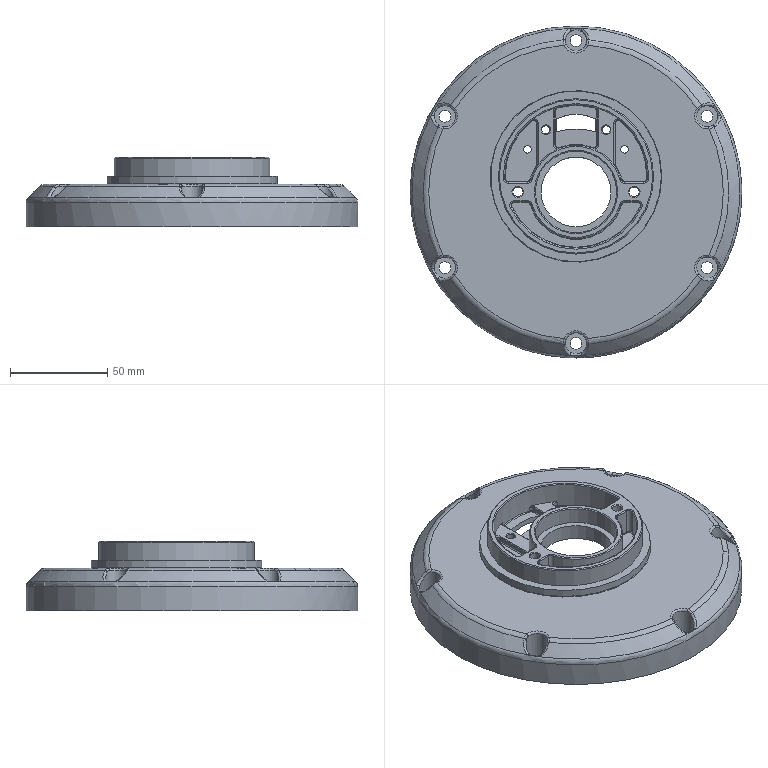NC program | NX | posted with a generic post | part box 171 x 171 x 36 mm
Lines 26826 to 27758 of 127321:
(3D开粗_COPY_COPY , TOOL : D4-L24)
N53638 T08 M6
N53640 G54
N53642 G17 G0 G90 X-30.607 Y7.686 S5000 M3
N53644 G43 Z20. H8
N53646 Z0.152
N53648 G94 G1 Z-0.148 F2500.
N53650 Y7.65
N53652 G3 X-30.007 Y7.05 R0.6
N53654 G1 X-25.078
N53656 G2 X25.078 Y7.05 R26.05
N53658 G1 X34.937
N53660 G3 X-34.937 Y7.05 R-34.95
N53662 G1 X-30.007
N53664 X-29.507
N53666 G3 X-28.907 Y7.65 R0.6
N53668 G1 Y7.686
N53670 Z0.152
N53672 X-30.607 Y7.74 Z0.004 F15000.
N53674 Z-0.296 F2500.
N53676 Y7.725
N53678 G3 X-30.007 Y7.125 R0.6
N53680 G1 X-25.135
N53682 G2 X25.135 Y7.125 R26.125
N53684 G1 X34.864
N53686 G3 X-34.864 Y7.125 R-34.875
N53688 G1 X-30.007
N53690 X-29.507
N53692 G3 X-28.907 Y7.73 R0.6
N53694 G1 Z0.004
N53696 G0 Z20.
N53698 X33.428 Y7.757
N53700 Z-0.144
N53702 G1 Z-0.444
N53704 G3 X34.028 Y7.157 R0.6
N53706 G1 X34.832
N53708 G3 X34.843 Y7.974 R34.843
N53710 X34.238 Y8.574 R0.6
N53712 G1 Z-0.144
N53714 X33.441 Y7.76 Z-0.292 F15000.
N53716 Z-0.592 F2500.
N53718 G3 X34.041 Y7.16 R0.6
N53720 G1 X34.83
N53722 G3 X34.84 Y7.961 R34.84
N53724 X34.235 Y8.561 R0.6
N53726 G1 Z-0.292
N53728 X33.441 Y7.76 Z-0.44 F15000.
N53730 Z-0.74 F2500.
N53732 G3 X34.041 Y7.16 R0.6
N53734 G1 X34.83
N53736 G3 X34.84 Y7.961 R34.84
N53738 X34.235 Y8.561 R0.6
N53740 G1 Z-0.44
N53742 X33.441 Y7.76 Z-0.588 F15000.
N53744 Z-0.888 F2500.
N53746 G3 X34.041 Y7.16 R0.6
N53748 G1 X34.83
N53750 G3 X34.84 Y7.961 R34.84
N53752 X34.235 Y8.561 R0.6
N53754 G1 Z-0.588
N53756 X33.441 Y7.76 Z-0.736 F15000.
N53758 Z-1.036 F2500.
N53760 G3 X34.041 Y7.16 R0.6
N53762 G1 X34.83
N53764 G3 X34.84 Y7.961 R34.84
N53766 X34.235 Y8.561 R0.6
N53768 G1 Z-0.736
N53770 X33.441 Y7.76 Z-0.884 F15000.
N53772 Z-1.184 F2500.
N53774 G3 X34.041 Y7.16 R0.6
N53776 G1 X34.83
N53778 G3 X34.84 Y7.961 R34.84
N53780 X34.235 Y8.561 R0.6
N53782 G1 Z-0.884
N53784 X33.441 Y7.76 Z-1.032 F15000.
N53786 Z-1.332 F2500.
N53788 G3 X34.041 Y7.16 R0.6
N53790 G1 X34.83
N53792 G3 X34.84 Y7.961 R34.84
N53794 X34.235 Y8.561 R0.6
N53796 G1 Z-1.032
N53798 X33.441 Y7.76 Z-1.18 F15000.
N53800 Z-1.48 F2500.
N53802 G3 X34.041 Y7.16 R0.6
N53804 G1 X34.83
N53806 G3 X34.84 Y7.961 R34.84
N53808 X34.235 Y8.561 R0.6
N53810 G1 Z-1.18
N53812 X33.441 Y7.76 Z-1.328 F15000.
N53814 Z-1.628 F2500.
N53816 G3 X34.041 Y7.16 R0.6
N53818 G1 X34.83
N53820 G3 X34.84 Y7.961 R34.84
N53822 X34.235 Y8.561 R0.6
N53824 G1 Z-1.328
N53826 X33.441 Y7.76 Z-1.476 F15000.
N53828 Z-1.776 F2500.
N53830 G3 X34.041 Y7.16 R0.6
N53832 G1 X34.83
N53834 G3 X34.84 Y7.961 R34.84
N53836 X34.235 Y8.561 R0.6
N53838 G1 Z-1.476
N53840 X33.441 Y7.76 Z-1.624 F15000.
N53842 Z-1.924 F2500.
N53844 G3 X34.041 Y7.16 R0.6
N53846 G1 X34.83
N53848 G3 X34.84 Y7.961 R34.84
N53850 X34.235 Y8.561 R0.6
N53852 G1 Z-1.624
N53854 X33.441 Y7.76 Z-1.772 F15000.
N53856 Z-2.072 F2500.
N53858 G3 X34.041 Y7.16 R0.6
N53860 G1 X34.83
N53862 G3 X34.84 Y7.961 R34.84
N53864 X34.235 Y8.561 R0.6
N53866 G1 Z-1.772
N53868 X33.441 Y7.76 Z-1.92 F15000.
N53870 Z-2.22 F2500.
N53872 G3 X34.041 Y7.16 R0.6
N53874 G1 X34.83
N53876 G3 X34.84 Y7.961 R34.84
N53878 X34.235 Y8.561 R0.6
N53880 G1 Z-1.92
N53882 X33.441 Y7.76 Z-2.068 F15000.
N53884 Z-2.368 F2500.
N53886 G3 X34.041 Y7.16 R0.6
N53888 G1 X34.83
N53890 G3 X34.84 Y7.961 R34.84
N53892 X34.235 Y8.561 R0.6
N53894 G1 Z-2.068
N53896 X33.441 Y7.76 Z-2.216 F15000.
N53898 Z-2.516 F2500.
N53900 G3 X34.041 Y7.16 R0.6
N53902 G1 X34.83
N53904 G3 X34.84 Y7.961 R34.84
N53906 X34.235 Y8.561 R0.6
N53908 G1 Z-2.216
N53910 X33.441 Y7.76 Z-2.364 F15000.
N53912 Z-2.664 F2500.
N53914 G3 X34.041 Y7.16 R0.6
N53916 G1 X34.83
N53918 G3 X34.84 Y7.961 R34.84
N53920 X34.235 Y8.561 R0.6
N53922 G1 Z-2.364
N53924 X33.441 Y7.76 Z-2.512 F15000.
N53926 Z-2.812 F2500.
N53928 G3 X34.041 Y7.16 R0.6
N53930 G1 X34.83
N53932 G3 X34.84 Y7.961 R34.84
N53934 X34.235 Y8.561 R0.6
N53936 G1 Z-2.512
N53938 X33.441 Y7.76 Z-2.66 F15000.
N53940 Z-2.96 F2500.
N53942 G3 X34.041 Y7.16 R0.6
N53944 G1 X34.83
N53946 G3 X34.84 Y7.961 R34.84
N53948 X34.235 Y8.561 R0.6
N53950 G1 Z-2.66
N53952 X33.441 Y7.76 Z-2.808 F15000.
N53954 Z-3.108 F2500.
N53956 G3 X34.041 Y7.16 R0.6
N53958 G1 X34.83
N53960 G3 X34.84 Y7.961 R34.84
N53962 X34.235 Y8.561 R0.6
N53964 G1 Z-2.808
N53966 X33.441 Y7.76 Z-2.956 F15000.
N53968 Z-3.256 F2500.
N53970 G3 X34.041 Y7.16 R0.6
N53972 G1 X34.83
N53974 G3 X34.84 Y7.961 R34.84
N53976 X34.235 Y8.561 R0.6
N53978 G1 Z-2.956
N53980 X33.441 Y7.76 Z-3.104 F15000.
N53982 Z-3.404 F2500.
N53984 G3 X34.041 Y7.16 R0.6
N53986 G1 X34.83
N53988 G3 X34.84 Y7.961 R34.84
N53990 X34.235 Y8.561 R0.6
N53992 G1 Z-3.104
N53994 X33.441 Y7.76 Z-3.252 F15000.
N53996 Z-3.552 F2500.
N53998 G3 X34.041 Y7.16 R0.6
N54000 G1 X34.83
N54002 G3 X34.84 Y7.961 R34.84
N54004 X34.235 Y8.561 R0.6
N54006 G1 Z-3.252
N54008 X33.441 Y7.76 Z-3.4 F15000.
N54010 Z-3.7 F2500.
N54012 G3 X34.041 Y7.16 R0.6
N54014 G1 X34.83
N54016 G3 X34.84 Y7.961 R34.84
N54018 X34.235 Y8.561 R0.6
N54020 G1 Z-3.4
N54022 X33.441 Y7.76 Z-3.548 F15000.
N54024 Z-3.848 F2500.
N54026 G3 X34.041 Y7.16 R0.6
N54028 G1 X34.83
N54030 G3 X34.84 Y7.961 R34.84
N54032 X34.235 Y8.561 R0.6
N54034 G1 Z-3.548
N54036 X33.441 Y7.76 Z-3.696 F15000.
N54038 Z-3.996 F2500.
N54040 G3 X34.041 Y7.16 R0.6
N54042 G1 X34.83
N54044 G3 X34.84 Y7.961 R34.84
N54046 X34.235 Y8.561 R0.6
N54048 G1 Z-3.696
N54050 X33.441 Y7.76 Z-3.844 F15000.
N54052 Z-4.144 F2500.
N54054 G3 X34.041 Y7.16 R0.6
N54056 G1 X34.83
N54058 G3 X34.84 Y7.961 R34.84
N54060 X34.235 Y8.561 R0.6
N54062 G1 Z-3.844
N54064 X33.441 Y7.76 Z-3.992 F15000.
N54066 Z-4.292 F2500.
N54068 G3 X34.041 Y7.16 R0.6
N54070 G1 X34.83
N54072 G3 X34.84 Y7.961 R34.84
N54074 X34.235 Y8.561 R0.6
N54076 G1 Z-3.992
N54078 X33.441 Y7.76 Z-4.14 F15000.
N54080 Z-4.44 F2500.
N54082 G3 X34.041 Y7.16 R0.6
N54084 G1 X34.83
N54086 G3 X34.84 Y7.961 R34.84
N54088 X34.235 Y8.561 R0.6
N54090 G1 Z-4.14
N54092 X33.441 Y7.76 Z-4.288 F15000.
N54094 Z-4.588 F2500.
N54096 G3 X34.041 Y7.16 R0.6
N54098 G1 X34.83
N54100 G3 X34.84 Y7.961 R34.84
N54102 X34.235 Y8.561 R0.6
N54104 G1 Z-4.288
N54106 X33.441 Y7.76 Z-4.436 F15000.
N54108 Z-4.736 F2500.
N54110 G3 X34.041 Y7.16 R0.6
N54112 G1 X34.83
N54114 G3 X34.84 Y7.961 R34.84
N54116 X34.235 Y8.561 R0.6
N54118 G1 Z-4.436
N54120 X33.441 Y7.76 Z-4.584 F15000.
N54122 Z-4.884 F2500.
N54124 G3 X34.041 Y7.16 R0.6
N54126 G1 X34.83
N54128 G3 X34.84 Y7.961 R34.84
N54130 X34.235 Y8.561 R0.6
N54132 G1 Z-4.584
N54134 X33.441 Y7.76 Z-4.732 F15000.
N54136 Z-5.032 F2500.
N54138 G3 X34.041 Y7.16 R0.6
N54140 G1 X34.83
N54142 G3 X34.84 Y7.961 R34.84
N54144 X34.235 Y8.561 R0.6
N54146 G1 Z-4.732
N54148 X33.441 Y7.76 Z-4.88 F15000.
N54150 Z-5.18 F2500.
N54152 G3 X34.041 Y7.16 R0.6
N54154 G1 X34.83
N54156 G3 X34.84 Y7.961 R34.84
N54158 X34.235 Y8.561 R0.6
N54160 G1 Z-4.88
N54162 X33.441 Y7.76 Z-5.028 F15000.
N54164 Z-5.328 F2500.
N54166 G3 X34.041 Y7.16 R0.6
N54168 G1 X34.83
N54170 G3 X34.84 Y7.961 R34.84
N54172 X34.235 Y8.561 R0.6
N54174 G1 Z-5.028
N54176 X33.441 Y7.76 Z-5.176 F15000.
N54178 Z-5.476 F2500.
N54180 G3 X34.041 Y7.16 R0.6
N54182 G1 X34.83
N54184 G3 X34.84 Y7.961 R34.84
N54186 X34.235 Y8.561 R0.6
N54188 G1 Z-5.176
N54190 X33.441 Y7.76 Z-5.324 F15000.
N54192 Z-5.624 F2500.
N54194 G3 X34.041 Y7.16 R0.6
N54196 G1 X34.83
N54198 G3 X34.84 Y7.961 R34.84
N54200 X34.235 Y8.561 R0.6
N54202 G1 Z-5.324
N54204 X33.441 Y7.76 Z-5.472 F15000.
N54206 Z-5.772 F2500.
N54208 G3 X34.041 Y7.16 R0.6
N54210 G1 X34.83
N54212 G3 X34.84 Y7.961 R34.84
N54214 X34.235 Y8.561 R0.6
N54216 G1 Z-5.472
N54218 X33.441 Y7.76 Z-5.62 F15000.
N54220 Z-5.92 F2500.
N54222 G3 X34.041 Y7.16 R0.6
N54224 G1 X34.83
N54226 G3 X34.84 Y7.961 R34.84
N54228 X34.235 Y8.561 R0.6
N54230 G1 Z-5.62
N54232 X33.441 Y7.76 Z-5.768 F15000.
N54234 Z-6.068 F2500.
N54236 G3 X34.041 Y7.16 R0.6
N54238 G1 X34.83
N54240 G3 X34.84 Y7.961 R34.84
N54242 X34.235 Y8.561 R0.6
N54244 G1 Z-5.768
N54246 X33.441 Y7.76 Z-5.916 F15000.
N54248 Z-6.216 F2500.
N54250 G3 X34.041 Y7.16 R0.6
N54252 G1 X34.83
N54254 G3 X34.84 Y7.961 R34.84
N54256 X34.235 Y8.561 R0.6
N54258 G1 Z-5.916
N54260 X33.441 Y7.76 Z-6.064 F15000.
N54262 Z-6.364 F2500.
N54264 G3 X34.041 Y7.16 R0.6
N54266 G1 X34.83
N54268 G3 X34.84 Y7.961 R34.84
N54270 X34.235 Y8.561 R0.6
N54272 G1 Z-6.064
N54274 X33.441 Y7.76 Z-6.212 F15000.
N54276 Z-6.512 F2500.
N54278 G3 X34.041 Y7.16 R0.6
N54280 G1 X34.83
N54282 G3 X34.84 Y7.961 R34.84
N54284 X34.235 Y8.561 R0.6
N54286 G1 Z-6.212
N54288 X33.441 Y7.76 Z-6.36 F15000.
N54290 Z-6.66 F2500.
N54292 G3 X34.041 Y7.16 R0.6
N54294 G1 X34.83
N54296 G3 X34.84 Y7.961 R34.84
N54298 X34.235 Y8.561 R0.6
N54300 G1 Z-6.36
N54302 X33.441 Y7.76 Z-6.508 F15000.
N54304 Z-6.808 F2500.
N54306 G3 X34.041 Y7.16 R0.6
N54308 G1 X34.83
N54310 G3 X34.84 Y7.961 R34.84
N54312 X34.235 Y8.561 R0.6
N54314 G1 Z-6.508
N54316 X33.441 Y7.76 Z-6.656 F15000.
N54318 Z-6.956 F2500.
N54320 G3 X34.041 Y7.16 R0.6
N54322 G1 X34.83
N54324 G3 X34.84 Y7.961 R34.84
N54326 X34.235 Y8.561 R0.6
N54328 G1 Z-6.656
N54330 X33.441 Y7.76 Z-6.804 F15000.
N54332 Z-7.104 F2500.
N54334 G3 X34.041 Y7.16 R0.6
N54336 G1 X34.83
N54338 G3 X34.84 Y7.961 R34.84
N54340 X34.235 Y8.561 R0.6
N54342 G1 Z-6.804
N54344 X33.441 Y7.76 Z-6.952 F15000.
N54346 Z-7.252 F2500.
N54348 G3 X34.041 Y7.16 R0.6
N54350 G1 X34.83
N54352 G3 X34.84 Y7.961 R34.84
N54354 X34.235 Y8.561 R0.6
N54356 G1 Z-6.952
N54358 X33.441 Y7.76 Z-7.1 F15000.
N54360 Z-7.4 F2500.
N54362 G3 X34.041 Y7.16 R0.6
N54364 G1 X34.83
N54366 G3 X34.84 Y7.961 R34.84
N54368 X34.235 Y8.561 R0.6
N54370 G1 Z-7.1
N54372 X33.441 Y7.76 Z-7.248 F15000.
N54374 Z-7.548 F2500.
N54376 G3 X34.041 Y7.16 R0.6
N54378 G1 X34.83
N54380 G3 X34.84 Y7.961 R34.84
N54382 X34.235 Y8.561 R0.6
N54384 G1 Z-7.248
N54386 X33.441 Y7.76 Z-7.396 F15000.
N54388 Z-7.696 F2500.
N54390 G3 X34.041 Y7.16 R0.6
N54392 G1 X34.83
N54394 G3 X34.84 Y7.961 R34.84
N54396 X34.235 Y8.561 R0.6
N54398 G1 Z-7.396
N54400 X33.441 Y7.76 Z-7.544 F15000.
N54402 Z-7.844 F2500.
N54404 G3 X34.041 Y7.16 R0.6
N54406 G1 X34.83
N54408 G3 X34.84 Y7.961 R34.84
N54410 X34.235 Y8.561 R0.6
N54412 G1 Z-7.544
N54414 X33.441 Y7.76 Z-7.692 F15000.
N54416 Z-7.992 F2500.
N54418 G3 X34.041 Y7.16 R0.6
N54420 G1 X34.83
N54422 G3 X34.84 Y7.961 R34.84
N54424 X34.235 Y8.561 R0.6
N54426 G1 Z-7.692
N54428 X33.441 Y7.76 Z-7.84 F15000.
N54430 Z-8.14 F2500.
N54432 G3 X34.041 Y7.16 R0.6
N54434 G1 X34.83
N54436 G3 X34.84 Y7.961 R34.84
N54438 X34.235 Y8.561 R0.6
N54440 G1 Z-7.84
N54442 X33.441 Y7.76 Z-7.988 F15000.
N54444 Z-8.288 F2500.
N54446 G3 X34.041 Y7.16 R0.6
N54448 G1 X34.83
N54450 G3 X34.84 Y7.961 R34.84
N54452 X34.235 Y8.561 R0.6
N54454 G1 Z-7.988
N54456 X33.441 Y7.76 Z-8.136 F15000.
N54458 Z-8.436 F2500.
N54460 G3 X34.041 Y7.16 R0.6
N54462 G1 X34.83
N54464 G3 X34.84 Y7.961 R34.84
N54466 X34.235 Y8.561 R0.6
N54468 G1 Z-8.136
N54470 X33.441 Y7.76 Z-8.284 F15000.
N54472 Z-8.584 F2500.
N54474 G3 X34.041 Y7.16 R0.6
N54476 G1 X34.83
N54478 G3 X34.84 Y7.961 R34.84
N54480 X34.235 Y8.561 R0.6
N54482 G1 Z-8.284
N54484 X33.441 Y7.76 Z-8.432 F15000.
N54486 Z-8.732 F2500.
N54488 G3 X34.041 Y7.16 R0.6
N54490 G1 X34.83
N54492 G3 X34.84 Y7.961 R34.84
N54494 X34.235 Y8.561 R0.6
N54496 G1 Z-8.432
N54498 X33.441 Y7.76 Z-8.58 F15000.
N54500 Z-8.88 F2500.
N54502 G3 X34.041 Y7.16 R0.6
N54504 G1 X34.83
N54506 G3 X34.84 Y7.961 R34.84
N54508 X34.235 Y8.561 R0.6
N54510 G1 Z-8.58
N54512 X33.441 Y7.76 Z-8.723 F15000.
N54514 Z-9.023 F2500.
N54516 G3 X34.041 Y7.16 R0.6
N54518 G1 X34.83
N54520 G3 X34.84 Y7.961 R34.84
N54522 X34.235 Y8.561 R0.6
N54524 G1 Z-8.723
N54526 X33.441 Y7.76 Z-8.866 F15000.
N54528 Z-9.166 F2500.
N54530 G3 X34.041 Y7.16 R0.6
N54532 G1 X34.83
N54534 G3 X34.84 Y7.961 R34.84
N54536 X34.235 Y8.561 R0.6
N54538 G1 Z-8.866
N54540 X33.441 Y7.76 Z-9.009 F15000.
N54542 Z-9.309 F2500.
N54544 G3 X34.041 Y7.16 R0.6
N54546 G1 X34.83
N54548 G3 X34.84 Y7.961 R34.84
N54550 X34.235 Y8.561 R0.6
N54552 G1 Z-9.009
N54554 X33.441 Y7.76 Z-9.151 F15000.
N54556 Z-9.451 F2500.
N54558 G3 X34.041 Y7.16 R0.6
N54560 G1 X34.83
N54562 G3 X34.84 Y7.961 R34.84
N54564 X34.235 Y8.561 R0.6
N54566 G1 Z-9.151
N54568 X33.441 Y7.76 Z-9.294 F15000.
N54570 Z-9.594 F2500.
N54572 G3 X34.041 Y7.16 R0.6
N54574 G1 X34.83
N54576 G3 X34.84 Y7.961 R34.84
N54578 X34.235 Y8.561 R0.6
N54580 G1 Z-9.294
N54582 X33.441 Y7.76 Z-9.437 F15000.
N54584 Z-9.737 F2500.
N54586 G3 X34.041 Y7.16 R0.6
N54588 G1 X34.83
N54590 G3 X34.84 Y7.961 R34.84
N54592 X34.235 Y8.561 R0.6
N54594 G1 Z-9.437
N54596 X33.441 Y7.76 Z-9.58 F15000.
N54598 Z-9.88 F2500.
N54600 G3 X34.041 Y7.16 R0.6
N54602 G1 X34.83
N54604 G3 X34.84 Y7.961 R34.84
N54606 X34.235 Y8.561 R0.6
N54608 G1 Z-9.58
N54610 X33.441 Y7.76 Z-9.723 F15000.
N54612 Z-10.023 F2500.
N54614 G3 X34.041 Y7.16 R0.6
N54616 G1 X34.83
N54618 G3 X34.84 Y7.961 R34.84
N54620 X34.235 Y8.561 R0.6
N54622 G1 Z-9.723
N54624 X33.441 Y7.76 Z-9.866 F15000.
N54626 Z-10.166 F2500.
N54628 G3 X34.041 Y7.16 R0.6
N54630 G1 X34.83
N54632 G3 X34.84 Y7.961 R34.84
N54634 X34.235 Y8.561 R0.6
N54636 G1 Z-9.866
N54638 X33.441 Y7.76 Z-10.009 F15000.
N54640 Z-10.309 F2500.
N54642 G3 X34.041 Y7.16 R0.6
N54644 G1 X34.83
N54646 G3 X34.84 Y7.961 R34.84
N54648 X34.235 Y8.561 R0.6
N54650 G1 Z-10.009
N54652 X33.441 Y7.76 Z-10.151 F15000.
N54654 Z-10.451 F2500.
N54656 G3 X34.041 Y7.16 R0.6
N54658 G1 X34.83
N54660 G3 X34.84 Y7.961 R34.84
N54662 X34.235 Y8.561 R0.6
N54664 G1 Z-10.151
N54666 X33.441 Y7.76 Z-10.294 F15000.
N54668 Z-10.594 F2500.
N54670 G3 X34.041 Y7.16 R0.6
N54672 G1 X34.83
N54674 G3 X34.84 Y7.961 R34.84
N54676 X34.235 Y8.561 R0.6
N54678 G1 Z-10.294
N54680 X33.441 Y7.76 Z-10.437 F15000.
N54682 Z-10.737 F2500.
N54684 G3 X34.041 Y7.16 R0.6
N54686 G1 X34.83
N54688 G3 X34.84 Y7.961 R34.84
N54690 X34.235 Y8.561 R0.6
N54692 G1 Z-10.437
N54694 X33.441 Y7.76 Z-10.58 F15000.
N54696 Z-10.88 F2500.
N54698 G3 X34.041 Y7.16 R0.6
N54700 G1 X34.83
N54702 G3 X34.84 Y7.961 R34.84
N54704 X34.235 Y8.561 R0.6
N54706 G1 Z-10.58
N54708 X33.441 Y7.76 Z-10.73 F15000.
N54710 Z-11.03 F2500.
N54712 G3 X34.041 Y7.16 R0.6
N54714 G1 X34.83
N54716 G3 X34.84 Y7.961 R34.84
N54718 X34.235 Y8.561 R0.6
N54720 G1 Z-10.73
N54722 X33.441 Y7.76 Z-10.88 F15000.
N54724 Z-11.18 F2500.
N54726 G3 X34.041 Y7.16 R0.6
N54728 G1 X34.83
N54730 G3 X34.84 Y7.961 R34.84
N54732 X34.235 Y8.561 R0.6
N54734 G1 Z-10.88
N54736 X33.441 Y7.76 Z-11.03 F15000.
N54738 Z-11.33 F2500.
N54740 G3 X34.041 Y7.16 R0.6
N54742 G1 X34.83
N54744 G3 X34.84 Y7.961 R34.84
N54746 X34.235 Y8.561 R0.6
N54748 G1 Z-11.03
N54750 X33.441 Y7.76 Z-11.18 F15000.
N54752 Z-11.48 F2500.
N54754 G3 X34.041 Y7.16 R0.6
N54756 G1 X34.83
N54758 Y7.174
N54760 G3 X34.84 Y7.961 R34.84
N54762 X34.235 Y8.561 R0.6
N54764 G1 Z-11.18
N54766 X33.441 Y7.76 Z-11.33 F15000.
N54768 Z-11.63 F2500.
N54770 G3 X34.041 Y7.16 R0.6
N54772 G1 X34.83
N54774 Y7.186
N54776 G3 X34.84 Y7.961 R34.84
N54778 X34.235 Y8.561 R0.6
N54780 G1 Z-11.33
N54782 X33.441 Y7.76 Z-11.48 F15000.
N54784 Z-11.78 F2500.
N54786 G3 X34.041 Y7.16 R0.6
N54788 G1 X34.83
N54790 X34.831 Y7.201
N54792 G3 X34.84 Y7.961 R34.84
N54794 X34.235 Y8.561 R0.6
N54796 G1 Z-11.48
N54798 X33.441 Y7.76 Z-11.63 F15000.
N54800 Z-11.93 F2500.
N54802 G3 X34.041 Y7.16 R0.6
N54804 G1 X34.83
N54806 X34.831 Y7.219
N54808 G3 X34.84 Y7.961 R34.84
N54810 X34.235 Y8.561 R0.6
N54812 G1 Z-11.63
N54814 X33.441 Y7.76 Z-11.78 F15000.
N54816 Z-12.08 F2500.
N54818 G3 X34.041 Y7.16 R0.6
N54820 G1 X34.83
N54822 X34.832 Y7.233
N54824 G3 X34.84 Y7.961 R34.84
N54826 X34.235 Y8.561 R0.6
N54828 G1 Z-11.78
N54830 X33.441 Y7.76 Z-11.93 F15000.
N54832 Z-12.23 F2500.
N54834 G3 X34.041 Y7.16 R0.6
N54836 G1 X34.83
N54838 X34.832 Y7.248
N54840 G3 X34.84 Y7.961 R34.84
N54842 X34.235 Y8.561 R0.6
N54844 G1 Z-11.93
N54846 X33.441 Y7.76 Z-12.08 F15000.
N54848 Z-12.38 F2500.
N54850 G3 X34.041 Y7.16 R0.6
N54852 G1 X34.83
N54854 X34.832 Y7.255
N54856 G3 X34.84 Y7.961 R34.84
N54858 X34.235 Y8.561 R0.6
N54860 G1 Z-12.08
N54862 X33.441 Y7.76 Z-12.23 F15000.
N54864 Z-12.53 F2500.
N54866 G3 X34.041 Y7.16 R0.6
N54868 G1 X34.83
N54870 X34.832 Y7.273
N54872 G3 X34.84 Y7.961 R34.84
N54874 X34.235 Y8.561 R0.6
N54876 G1 Z-12.23
N54878 X33.441 Y7.76 Z-12.38 F15000.
N54880 Z-12.68 F2500.
N54882 G3 X34.041 Y7.16 R0.6
N54884 G1 X34.83
N54886 X34.833 Y7.284
N54888 G3 X34.84 Y7.961 R34.84
N54890 X34.235 Y8.561 R0.6
N54892 G1 Z-12.38
N54894 X33.441 Y7.76 Z-12.53 F15000.
N54896 Z-12.83 F2500.
N54898 G3 X34.041 Y7.16 R0.6
N54900 G1 X34.83
N54902 X34.833 Y7.304
N54904 G3 X34.84 Y7.961 R34.84
N54906 X34.235 Y8.561 R0.6
N54908 G1 Z-12.53
N54910 X33.441 Y7.76 Z-12.68 F15000.
N54912 Z-12.98 F2500.
N54914 G3 X34.041 Y7.16 R0.6
N54916 G1 X34.83
N54918 X34.833 Y7.315
N54920 G3 X34.84 Y7.961 R34.84
N54922 X34.235 Y8.561 R0.6
N54924 G1 Z-12.68
N54926 X33.441 Y7.76 Z-12.83 F15000.
N54928 Z-13.13 F2500.
N54930 G3 X34.041 Y7.16 R0.6
N54932 G1 X34.83
N54934 X34.833 Y7.327
N54936 G3 X34.84 Y7.961 R34.84
N54938 X34.235 Y8.561 R0.6
N54940 G1 Z-12.83
N54942 X33.441 Y7.76 Z-12.98 F15000.
N54944 Z-13.28 F2500.
N54946 G3 X34.041 Y7.16 R0.6
N54948 G1 X34.83
N54950 X34.834 Y7.347
N54952 G3 X34.84 Y7.961 R34.84
N54954 X34.235 Y8.561 R0.6
N54956 G1 Z-12.98
N54958 G0 Z2.704
N54960 G1 X25.395 Y8.43 F15000.
N54962 G0 Z-0.144
N54964 G1 Z-0.444 F2500.
N54966 G3 X25.004 Y7.682 R0.6
N54968 G2 X25.159 Y7.157 R26.157
N54970 G1 X25.717
N54972 G3 X26.317 Y7.757 R0.6
N54974 G1 Z-0.144
N54976 X25.401 Y8.419 Z-0.292 F15000.
N54978 Z-0.592 F2500.
N54980 G3 X25.01 Y7.671 R0.6
N54982 G2 X25.161 Y7.16 R26.16
N54984 G1 X25.704
N54986 G3 X26.304 Y7.76 R0.6
N54988 G1 Z-0.292
N54990 X25.401 Y8.419 Z-0.44 F15000.
N54992 Z-0.74 F2500.
N54994 G3 X25.01 Y7.671 R0.6
N54996 G2 X25.161 Y7.16 R26.16
N54998 G1 X25.704
N55000 G3 X26.304 Y7.76 R0.6
N55002 G1 Z-0.44
N55004 X25.401 Y8.419 Z-0.588 F15000.
N55006 Z-0.888 F2500.
N55008 G3 X25.01 Y7.671 R0.6
N55010 G2 X25.161 Y7.16 R26.16
N55012 G1 X25.704
N55014 G3 X26.304 Y7.76 R0.6
N55016 G1 Z-0.588
N55018 X25.401 Y8.419 Z-0.736 F15000.
N55020 Z-1.036 F2500.
N55022 G3 X25.01 Y7.671 R0.6
N55024 G2 X25.161 Y7.16 R26.16
N55026 G1 X25.704
N55028 G3 X26.304 Y7.76 R0.6
N55030 G1 Z-0.736
N55032 X25.401 Y8.419 Z-0.884 F15000.
N55034 Z-1.184 F2500.
N55036 G3 X25.01 Y7.671 R0.6
N55038 G2 X25.161 Y7.16 R26.16
N55040 G1 X25.704
N55042 G3 X26.304 Y7.76 R0.6
N55044 G1 Z-0.884
N55046 X25.401 Y8.419 Z-1.032 F15000.
N55048 Z-1.332 F2500.
N55050 G3 X25.01 Y7.671 R0.6
N55052 G2 X25.161 Y7.16 R26.16
N55054 G1 X25.704
N55056 G3 X26.304 Y7.76 R0.6
N55058 G1 Z-1.032
N55060 X25.401 Y8.419 Z-1.18 F15000.
N55062 Z-1.48 F2500.
N55064 G3 X25.01 Y7.671 R0.6
N55066 G2 X25.161 Y7.16 R26.16
N55068 G1 X25.704
N55070 G3 X26.304 Y7.76 R0.6
N55072 G1 Z-1.18
N55074 X25.401 Y8.419 Z-1.328 F15000.
N55076 Z-1.628 F2500.
N55078 G3 X25.01 Y7.671 R0.6
N55080 G2 X25.161 Y7.16 R26.16
N55082 G1 X25.704
N55084 G3 X26.304 Y7.76 R0.6
N55086 G1 Z-1.328
N55088 X25.401 Y8.419 Z-1.476 F15000.
N55090 Z-1.776 F2500.
N55092 G3 X25.01 Y7.671 R0.6
N55094 G2 X25.161 Y7.16 R26.16
N55096 G1 X25.704
N55098 G3 X26.304 Y7.76 R0.6
N55100 G1 Z-1.476
N55102 X25.401 Y8.419 Z-1.624 F15000.
N55104 Z-1.924 F2500.
N55106 G3 X25.01 Y7.671 R0.6
N55108 G2 X25.161 Y7.16 R26.16
N55110 G1 X25.704
N55112 G3 X26.304 Y7.76 R0.6
N55114 G1 Z-1.624
N55116 X25.401 Y8.419 Z-1.772 F15000.
N55118 Z-2.072 F2500.
N55120 G3 X25.01 Y7.671 R0.6
N55122 G2 X25.161 Y7.16 R26.16
N55124 G1 X25.704
N55126 G3 X26.304 Y7.76 R0.6
N55128 G1 Z-1.772
N55130 X25.401 Y8.419 Z-1.92 F15000.
N55132 Z-2.22 F2500.
N55134 G3 X25.01 Y7.671 R0.6
N55136 G2 X25.161 Y7.16 R26.16
N55138 G1 X25.704
N55140 G3 X26.304 Y7.76 R0.6
N55142 G1 Z-1.92
N55144 X25.401 Y8.419 Z-2.068 F15000.
N55146 Z-2.368 F2500.
N55148 G3 X25.01 Y7.671 R0.6
N55150 G2 X25.161 Y7.16 R26.16
N55152 G1 X25.704
N55154 G3 X26.304 Y7.76 R0.6
N55156 G1 Z-2.068
N55158 X25.401 Y8.419 Z-2.216 F15000.
N55160 Z-2.516 F2500.
N55162 G3 X25.01 Y7.671 R0.6
N55164 G2 X25.161 Y7.16 R26.16
N55166 G1 X25.704
N55168 G3 X26.304 Y7.76 R0.6
N55170 G1 Z-2.216
N55172 X25.401 Y8.419 Z-2.364 F15000.
N55174 Z-2.664 F2500.
N55176 G3 X25.01 Y7.671 R0.6
N55178 G2 X25.161 Y7.16 R26.16
N55180 G1 X25.704
N55182 G3 X26.304 Y7.76 R0.6
N55184 G1 Z-2.364
N55186 X25.401 Y8.419 Z-2.512 F15000.
N55188 Z-2.812 F2500.
N55190 G3 X25.01 Y7.671 R0.6
N55192 G2 X25.161 Y7.16 R26.16
N55194 G1 X25.704
N55196 G3 X26.304 Y7.76 R0.6
N55198 G1 Z-2.512
N55200 X25.401 Y8.419 Z-2.66 F15000.
N55202 Z-2.96 F2500.
N55204 G3 X25.01 Y7.671 R0.6
N55206 G2 X25.161 Y7.16 R26.16
N55208 G1 X25.704
N55210 G3 X26.304 Y7.76 R0.6
N55212 G1 Z-2.66
N55214 X25.401 Y8.419 Z-2.808 F15000.
N55216 Z-3.108 F2500.
N55218 G3 X25.01 Y7.671 R0.6
N55220 G2 X25.161 Y7.16 R26.16
N55222 G1 X25.704
N55224 G3 X26.304 Y7.76 R0.6
N55226 G1 Z-2.808
N55228 X25.401 Y8.419 Z-2.956 F15000.
N55230 Z-3.256 F2500.
N55232 G3 X25.01 Y7.671 R0.6
N55234 G2 X25.161 Y7.16 R26.16
N55236 G1 X25.704
N55238 G3 X26.304 Y7.76 R0.6
N55240 G1 Z-2.956
N55242 X25.401 Y8.419 Z-3.104 F15000.
N55244 Z-3.404 F2500.
N55246 G3 X25.01 Y7.671 R0.6
N55248 G2 X25.161 Y7.16 R26.16
N55250 G1 X25.704
N55252 G3 X26.304 Y7.76 R0.6
N55254 G1 Z-3.104
N55256 X25.401 Y8.419 Z-3.252 F15000.
N55258 Z-3.552 F2500.
N55260 G3 X25.01 Y7.671 R0.6
N55262 G2 X25.161 Y7.16 R26.16
N55264 G1 X25.704
N55266 G3 X26.304 Y7.76 R0.6
N55268 G1 Z-3.252
N55270 X25.401 Y8.419 Z-3.4 F15000.
N55272 Z-3.7 F2500.
N55274 G3 X25.01 Y7.671 R0.6
N55276 G2 X25.161 Y7.16 R26.16
N55278 G1 X25.704
N55280 G3 X26.304 Y7.76 R0.6
N55282 G1 Z-3.4
N55284 X25.401 Y8.419 Z-3.548 F15000.
N55286 Z-3.848 F2500.
N55288 G3 X25.01 Y7.671 R0.6
N55290 G2 X25.161 Y7.16 R26.16
N55292 G1 X25.704
N55294 G3 X26.304 Y7.76 R0.6
N55296 G1 Z-3.548
N55298 X25.401 Y8.419 Z-3.696 F15000.
N55300 Z-3.996 F2500.
N55302 G3 X25.01 Y7.671 R0.6
N55304 G2 X25.161 Y7.16 R26.16
N55306 G1 X25.704
N55308 G3 X26.304 Y7.76 R0.6
N55310 G1 Z-3.696
N55312 X25.401 Y8.419 Z-3.844 F15000.
N55314 Z-4.144 F2500.
N55316 G3 X25.01 Y7.671 R0.6
N55318 G2 X25.161 Y7.16 R26.16
N55320 G1 X25.704
N55322 G3 X26.304 Y7.76 R0.6
N55324 G1 Z-3.844
N55326 X25.401 Y8.419 Z-3.992 F15000.
N55328 Z-4.292 F2500.
N55330 G3 X25.01 Y7.671 R0.6
N55332 G2 X25.161 Y7.16 R26.16
N55334 G1 X25.704
N55336 G3 X26.304 Y7.76 R0.6
N55338 G1 Z-3.992
N55340 X25.401 Y8.419 Z-4.14 F15000.
N55342 Z-4.44 F2500.
N55344 G3 X25.01 Y7.671 R0.6
N55346 G2 X25.161 Y7.16 R26.16
N55348 G1 X25.704
N55350 G3 X26.304 Y7.76 R0.6
N55352 G1 Z-4.14
N55354 X25.401 Y8.419 Z-4.288 F15000.
N55356 Z-4.588 F2500.
N55358 G3 X25.01 Y7.671 R0.6
N55360 G2 X25.161 Y7.16 R26.16
N55362 G1 X25.704
N55364 G3 X26.304 Y7.76 R0.6
N55366 G1 Z-4.288
N55368 X25.401 Y8.419 Z-4.436 F15000.
N55370 Z-4.736 F2500.
N55372 G3 X25.01 Y7.671 R0.6
N55374 G2 X25.161 Y7.16 R26.16
N55376 G1 X25.704
N55378 G3 X26.304 Y7.76 R0.6
N55380 G1 Z-4.436
N55382 X25.401 Y8.419 Z-4.584 F15000.
N55384 Z-4.884 F2500.
N55386 G3 X25.01 Y7.671 R0.6
N55388 G2 X25.161 Y7.16 R26.16
N55390 G1 X25.704
N55392 G3 X26.304 Y7.76 R0.6
N55394 G1 Z-4.584
N55396 X25.401 Y8.419 Z-4.732 F15000.
N55398 Z-5.032 F2500.
N55400 G3 X25.01 Y7.671 R0.6
N55402 G2 X25.161 Y7.16 R26.16
N55404 G1 X25.704
N55406 G3 X26.304 Y7.76 R0.6
N55408 G1 Z-4.732
N55410 X25.401 Y8.419 Z-4.88 F15000.
N55412 Z-5.18 F2500.
N55414 G3 X25.01 Y7.671 R0.6
N55416 G2 X25.161 Y7.16 R26.16
N55418 G1 X25.704
N55420 G3 X26.304 Y7.76 R0.6
N55422 G1 Z-4.88
N55424 X25.401 Y8.419 Z-5.028 F15000.
N55426 Z-5.328 F2500.
N55428 G3 X25.01 Y7.671 R0.6
N55430 G2 X25.161 Y7.16 R26.16
N55432 G1 X25.704
N55434 G3 X26.304 Y7.76 R0.6
N55436 G1 Z-5.028
N55438 X25.401 Y8.419 Z-5.176 F15000.
N55440 Z-5.476 F2500.
N55442 G3 X25.01 Y7.671 R0.6
N55444 G2 X25.161 Y7.16 R26.16
N55446 G1 X25.704
N55448 G3 X26.304 Y7.76 R0.6
N55450 G1 Z-5.176
N55452 X25.401 Y8.419 Z-5.324 F15000.
N55454 Z-5.624 F2500.
N55456 G3 X25.01 Y7.671 R0.6
N55458 G2 X25.161 Y7.16 R26.16
N55460 G1 X25.704
N55462 G3 X26.304 Y7.76 R0.6
N55464 G1 Z-5.324
N55466 X25.401 Y8.419 Z-5.472 F15000.
N55468 Z-5.772 F2500.
N55470 G3 X25.01 Y7.671 R0.6
N55472 G2 X25.161 Y7.16 R26.16
N55474 G1 X25.704
N55476 G3 X26.304 Y7.76 R0.6
N55478 G1 Z-5.472
N55480 X25.401 Y8.419 Z-5.62 F15000.
N55482 Z-5.92 F2500.
N55484 G3 X25.01 Y7.671 R0.6
N55486 G2 X25.161 Y7.16 R26.16
N55488 G1 X25.704
N55490 G3 X26.304 Y7.76 R0.6
N55492 G1 Z-5.62
N55494 X25.401 Y8.419 Z-5.768 F15000.
N55496 Z-6.068 F2500.